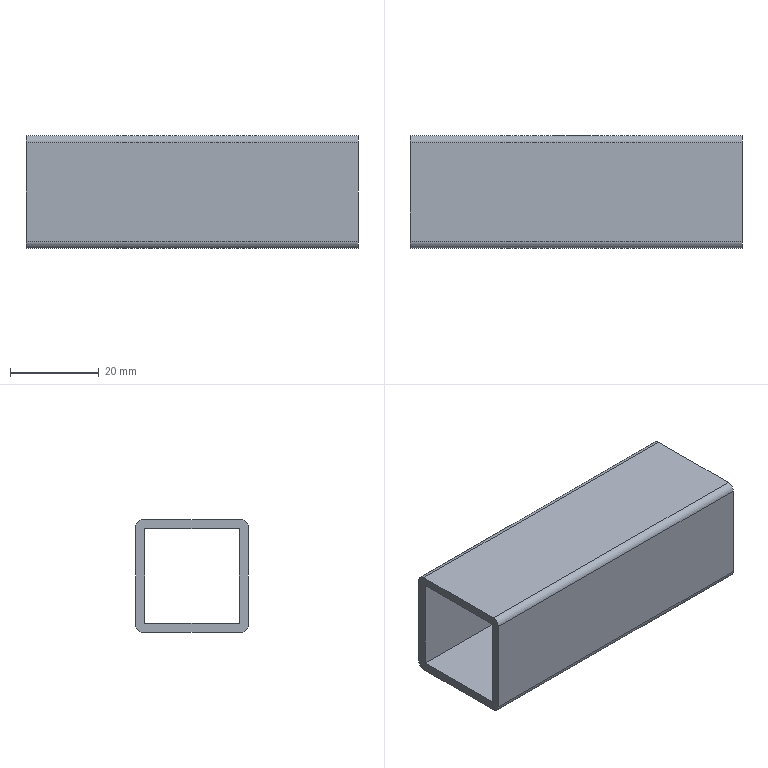Part | NX | features BREP 1 | 1 solid | 16 faces | box 74.93 x 25.4 x 25.4 mm | volume 13599 mm3 | plane 10 | cylinder 6 | commonest cylinder face diameters 3.175 x4 9.652 x2
STEP:
#1=CARTESIAN_POINT('',(-37.465,12.7,-11.113));
#2=VERTEX_POINT('',#1);
#3=CARTESIAN_POINT('',(-37.465,12.7,11.113));
#4=VERTEX_POINT('',#3);
#5=CARTESIAN_POINT('',(-37.465,12.7,-11.113));
#6=DIRECTION('',(0.,0.,1.));
#7=VECTOR('',#6,1000.);
#8=LINE('',#5,#7);
#9=EDGE_CURVE('',#2,#4,#8,.T.);
#10=ORIENTED_EDGE('',*,*,#9,.F.);
#11=CARTESIAN_POINT('',(-37.465,11.113,-12.7));
#12=VERTEX_POINT('',#11);
#13=CARTESIAN_POINT('',(-37.465,11.113,-11.113));
#14=DIRECTION('',(-1.,0.,0.));
#15=DIRECTION('',(0.,1.,0.));
#16=AXIS2_PLACEMENT_3D('',#13,#14,#15);
#17=CIRCLE('',#16,1.587);
#18=EDGE_CURVE('',#2,#12,#17,.T.);
#19=ORIENTED_EDGE('',*,*,#18,.T.);
#20=CARTESIAN_POINT('',(-37.465,-11.113,-12.7));
#21=VERTEX_POINT('',#20);
#22=CARTESIAN_POINT('',(-37.465,-11.113,-12.7));
#23=DIRECTION('',(0.,1.,0.));
#24=VECTOR('',#23,1000.);
#25=LINE('',#22,#24);
#26=EDGE_CURVE('',#21,#12,#25,.T.);
#27=ORIENTED_EDGE('',*,*,#26,.F.);
#28=CARTESIAN_POINT('',(-37.465,-12.7,-11.113));
#29=VERTEX_POINT('',#28);
#30=CARTESIAN_POINT('',(-37.465,-11.113,-11.113));
#31=DIRECTION('',(-1.,0.,0.));
#32=DIRECTION('',(0.,0.,-1.));
#33=AXIS2_PLACEMENT_3D('',#30,#31,#32);
#34=CIRCLE('',#33,1.587);
#35=EDGE_CURVE('',#21,#29,#34,.T.);
#36=ORIENTED_EDGE('',*,*,#35,.T.);
#37=CARTESIAN_POINT('',(-37.465,-12.7,11.113));
#38=VERTEX_POINT('',#37);
#39=CARTESIAN_POINT('',(-37.465,-12.7,11.113));
#40=DIRECTION('',(0.,0.,-1.));
#41=VECTOR('',#40,1000.);
#42=LINE('',#39,#41);
#43=EDGE_CURVE('',#38,#29,#42,.T.);
#44=ORIENTED_EDGE('',*,*,#43,.F.);
#45=CARTESIAN_POINT('',(-37.465,-11.113,12.7));
#46=VERTEX_POINT('',#45);
#47=CARTESIAN_POINT('',(-37.465,-11.113,11.113));
#48=DIRECTION('',(-1.,0.,0.));
#49=DIRECTION('',(0.,-1.,0.));
#50=AXIS2_PLACEMENT_3D('',#47,#48,#49);
#51=CIRCLE('',#50,1.587);
#52=EDGE_CURVE('',#38,#46,#51,.T.);
#53=ORIENTED_EDGE('',*,*,#52,.T.);
#54=CARTESIAN_POINT('',(-37.465,11.113,12.7));
#55=VERTEX_POINT('',#54);
#56=CARTESIAN_POINT('',(-37.465,11.113,12.7));
#57=DIRECTION('',(0.,-1.,0.));
#58=VECTOR('',#57,1000.);
#59=LINE('',#56,#58);
#60=EDGE_CURVE('',#55,#46,#59,.T.);
#61=ORIENTED_EDGE('',*,*,#60,.F.);
#62=CARTESIAN_POINT('',(-37.465,11.113,11.113));
#63=DIRECTION('',(-1.,0.,0.));
#64=DIRECTION('',(0.,0.,1.));
#65=AXIS2_PLACEMENT_3D('',#62,#63,#64);
#66=CIRCLE('',#65,1.587);
#67=EDGE_CURVE('',#55,#4,#66,.T.);
#68=ORIENTED_EDGE('',*,*,#67,.T.);
#69=EDGE_LOOP('',(#10,#19,#27,#36,#44,#53,#61,#68));
#70=FACE_BOUND('',#69,.T.);
#71=CARTESIAN_POINT('',(-37.465,10.719,10.719));
#72=VERTEX_POINT('',#71);
#73=CARTESIAN_POINT('',(-37.465,10.719,-10.719));
#74=VERTEX_POINT('',#73);
#75=CARTESIAN_POINT('',(-37.465,10.719,10.719));
#76=DIRECTION('',(0.,0.,-1.));
#77=VECTOR('',#76,1000.);
#78=LINE('',#75,#77);
#79=EDGE_CURVE('',#72,#74,#78,.T.);
#80=ORIENTED_EDGE('',*,*,#79,.F.);
#81=CARTESIAN_POINT('',(-37.465,-10.719,10.719));
#82=VERTEX_POINT('',#81);
#83=CARTESIAN_POINT('',(-37.465,-10.719,10.719));
#84=DIRECTION('',(0.,1.,0.));
#85=VECTOR('',#84,1000.);
#86=LINE('',#83,#85);
#87=EDGE_CURVE('',#82,#72,#86,.T.);
#88=ORIENTED_EDGE('',*,*,#87,.F.);
#89=CARTESIAN_POINT('',(-37.465,-10.719,-10.719));
#90=VERTEX_POINT('',#89);
#91=CARTESIAN_POINT('',(-37.465,-10.719,-10.719));
#92=DIRECTION('',(0.,0.,1.));
#93=VECTOR('',#92,1000.);
#94=LINE('',#91,#93);
#95=EDGE_CURVE('',#90,#82,#94,.T.);
#96=ORIENTED_EDGE('',*,*,#95,.F.);
#97=CARTESIAN_POINT('',(-37.465,10.719,-10.719));
#98=DIRECTION('',(0.,-1.,0.));
#99=VECTOR('',#98,1000.);
#100=LINE('',#97,#99);
#101=EDGE_CURVE('',#74,#90,#100,.T.);
#102=ORIENTED_EDGE('',*,*,#101,.F.);
#103=EDGE_LOOP('',(#80,#88,#96,#102));
#104=FACE_BOUND('',#103,.T.);
#105=CARTESIAN_POINT('',(-37.465,0.,0.));
#106=DIRECTION('',(1.,0.,0.));
#107=DIRECTION('',(0.,1.,0.));
#108=AXIS2_PLACEMENT_3D('',#105,#106,#107);
#109=PLANE('',#108);
#110=ADVANCED_FACE('',(#70,#104),#109,.F.);
#111=CARTESIAN_POINT('',(37.465,-10.719,-10.719));
#112=VERTEX_POINT('',#111);
#113=CARTESIAN_POINT('',(-37.465,-10.719,-10.719));
#114=DIRECTION('',(1.,0.,0.));
#115=VECTOR('',#114,1000.);
#116=LINE('',#113,#115);
#117=EDGE_CURVE('',#90,#112,#116,.T.);
#118=ORIENTED_EDGE('',*,*,#117,.T.);
#119=CARTESIAN_POINT('',(37.465,10.719,-10.719));
#120=VERTEX_POINT('',#119);
#121=CARTESIAN_POINT('',(37.465,10.719,-10.719));
#122=DIRECTION('',(0.,-1.,0.));
#123=VECTOR('',#122,1000.);
#124=LINE('',#121,#123);
#125=EDGE_CURVE('',#120,#112,#124,.T.);
#126=ORIENTED_EDGE('',*,*,#125,.F.);
#127=CARTESIAN_POINT('',(-37.465,10.719,-10.719));
#128=DIRECTION('',(1.,0.,0.));
#129=VECTOR('',#128,1000.);
#130=LINE('',#127,#129);
#131=EDGE_CURVE('',#74,#120,#130,.T.);
#132=ORIENTED_EDGE('',*,*,#131,.F.);
#133=ORIENTED_EDGE('',*,*,#101,.T.);
#134=EDGE_LOOP('',(#118,#126,#132,#133));
#135=FACE_BOUND('',#134,.T.);
#136=CARTESIAN_POINT('',(-37.465,10.719,-10.719));
#137=DIRECTION('',(0.,0.,1.));
#138=DIRECTION('',(1.,0.,0.));
#139=AXIS2_PLACEMENT_3D('',#136,#137,#138);
#140=PLANE('',#139);
#141=ADVANCED_FACE('',(#135),#140,.T.);
#142=ORIENTED_EDGE('',*,*,#131,.T.);
#143=CARTESIAN_POINT('',(37.465,10.719,10.719));
#144=VERTEX_POINT('',#143);
#145=CARTESIAN_POINT('',(37.465,10.719,10.719));
#146=DIRECTION('',(0.,0.,-1.));
#147=VECTOR('',#146,1000.);
#148=LINE('',#145,#147);
#149=EDGE_CURVE('',#144,#120,#148,.T.);
#150=ORIENTED_EDGE('',*,*,#149,.F.);
#151=CARTESIAN_POINT('',(-37.465,10.719,10.719));
#152=DIRECTION('',(1.,0.,0.));
#153=VECTOR('',#152,1000.);
#154=LINE('',#151,#153);
#155=EDGE_CURVE('',#72,#144,#154,.T.);
#156=ORIENTED_EDGE('',*,*,#155,.F.);
#157=ORIENTED_EDGE('',*,*,#79,.T.);
#158=EDGE_LOOP('',(#142,#150,#156,#157));
#159=FACE_BOUND('',#158,.T.);
#160=CARTESIAN_POINT('',(-4.826,10.719,0.));
#161=VERTEX_POINT('',#160);
#162=CARTESIAN_POINT('',(4.826,10.719,0.));
#163=VERTEX_POINT('',#162);
#164=CARTESIAN_POINT('',(0.,10.719,0.));
#165=DIRECTION('',(0.,-1.,0.));
#166=DIRECTION('',(-1.,0.,0.));
#167=AXIS2_PLACEMENT_3D('',#164,#165,#166);
#168=CIRCLE('',#167,4.826);
#169=EDGE_CURVE('',#161,#163,#168,.T.);
#170=ORIENTED_EDGE('',*,*,#169,.F.);
#171=CARTESIAN_POINT('',(0.,10.719,0.));
#172=DIRECTION('',(0.,-1.,0.));
#173=DIRECTION('',(1.,0.,0.));
#174=AXIS2_PLACEMENT_3D('',#171,#172,#173);
#175=CIRCLE('',#174,4.826);
#176=EDGE_CURVE('',#163,#161,#175,.T.);
#177=ORIENTED_EDGE('',*,*,#176,.F.);
#178=EDGE_LOOP('',(#170,#177));
#179=FACE_BOUND('',#178,.T.);
#180=CARTESIAN_POINT('',(-37.465,10.719,10.719));
#181=DIRECTION('',(0.,-1.,0.));
#182=DIRECTION('',(0.,0.,-1.));
#183=AXIS2_PLACEMENT_3D('',#180,#181,#182);
#184=PLANE('',#183);
#185=ADVANCED_FACE('',(#159,#179),#184,.T.);
#186=ORIENTED_EDGE('',*,*,#155,.T.);
#187=CARTESIAN_POINT('',(37.465,-10.719,10.719));
#188=VERTEX_POINT('',#187);
#189=CARTESIAN_POINT('',(37.465,-10.719,10.719));
#190=DIRECTION('',(0.,1.,0.));
#191=VECTOR('',#190,1000.);
#192=LINE('',#189,#191);
#193=EDGE_CURVE('',#188,#144,#192,.T.);
#194=ORIENTED_EDGE('',*,*,#193,.F.);
#195=CARTESIAN_POINT('',(-37.465,-10.719,10.719));
#196=DIRECTION('',(1.,0.,0.));
#197=VECTOR('',#196,1000.);
#198=LINE('',#195,#197);
#199=EDGE_CURVE('',#82,#188,#198,.T.);
#200=ORIENTED_EDGE('',*,*,#199,.F.);
#201=ORIENTED_EDGE('',*,*,#87,.T.);
#202=EDGE_LOOP('',(#186,#194,#200,#201));
#203=FACE_BOUND('',#202,.T.);
#204=CARTESIAN_POINT('',(-37.465,-10.719,10.719));
#205=DIRECTION('',(0.,0.,-1.));
#206=DIRECTION('',(0.,-1.,0.));
#207=AXIS2_PLACEMENT_3D('',#204,#205,#206);
#208=PLANE('',#207);
#209=ADVANCED_FACE('',(#203),#208,.T.);
#210=ORIENTED_EDGE('',*,*,#199,.T.);
#211=CARTESIAN_POINT('',(37.465,-10.719,-10.719));
#212=DIRECTION('',(0.,0.,1.));
#213=VECTOR('',#212,1000.);
#214=LINE('',#211,#213);
#215=EDGE_CURVE('',#112,#188,#214,.T.);
#216=ORIENTED_EDGE('',*,*,#215,.F.);
#217=ORIENTED_EDGE('',*,*,#117,.F.);
#218=ORIENTED_EDGE('',*,*,#95,.T.);
#219=EDGE_LOOP('',(#210,#216,#217,#218));
#220=FACE_BOUND('',#219,.T.);
#221=CARTESIAN_POINT('',(-37.465,-10.719,-10.719));
#222=DIRECTION('',(0.,1.,0.));
#223=DIRECTION('',(1.,0.,0.));
#224=AXIS2_PLACEMENT_3D('',#221,#222,#223);
#225=PLANE('',#224);
#226=ADVANCED_FACE('',(#220),#225,.T.);
#227=CARTESIAN_POINT('',(37.465,11.113,12.7));
#228=VERTEX_POINT('',#227);
#229=CARTESIAN_POINT('',(37.465,-11.113,12.7));
#230=VERTEX_POINT('',#229);
#231=CARTESIAN_POINT('',(37.465,11.113,12.7));
#232=DIRECTION('',(0.,-1.,0.));
#233=VECTOR('',#232,1000.);
#234=LINE('',#231,#233);
#235=EDGE_CURVE('',#228,#230,#234,.T.);
#236=ORIENTED_EDGE('',*,*,#235,.T.);
#237=CARTESIAN_POINT('',(37.465,-12.7,11.113));
#238=VERTEX_POINT('',#237);
#239=CARTESIAN_POINT('',(37.465,-11.113,11.113));
#240=DIRECTION('',(1.,0.,0.));
#241=DIRECTION('',(0.,0.,1.));
#242=AXIS2_PLACEMENT_3D('',#239,#240,#241);
#243=CIRCLE('',#242,1.587);
#244=EDGE_CURVE('',#230,#238,#243,.T.);
#245=ORIENTED_EDGE('',*,*,#244,.T.);
#246=CARTESIAN_POINT('',(37.465,-12.7,-11.113));
#247=VERTEX_POINT('',#246);
#248=CARTESIAN_POINT('',(37.465,-12.7,11.113));
#249=DIRECTION('',(0.,0.,-1.));
#250=VECTOR('',#249,1000.);
#251=LINE('',#248,#250);
#252=EDGE_CURVE('',#238,#247,#251,.T.);
#253=ORIENTED_EDGE('',*,*,#252,.T.);
#254=CARTESIAN_POINT('',(37.465,-11.113,-12.7));
#255=VERTEX_POINT('',#254);
#256=CARTESIAN_POINT('',(37.465,-11.113,-11.113));
#257=DIRECTION('',(1.,0.,0.));
#258=DIRECTION('',(0.,-1.,0.));
#259=AXIS2_PLACEMENT_3D('',#256,#257,#258);
#260=CIRCLE('',#259,1.587);
#261=EDGE_CURVE('',#247,#255,#260,.T.);
#262=ORIENTED_EDGE('',*,*,#261,.T.);
#263=CARTESIAN_POINT('',(37.465,11.113,-12.7));
#264=VERTEX_POINT('',#263);
#265=CARTESIAN_POINT('',(37.465,-11.113,-12.7));
#266=DIRECTION('',(0.,1.,0.));
#267=VECTOR('',#266,1000.);
#268=LINE('',#265,#267);
#269=EDGE_CURVE('',#255,#264,#268,.T.);
#270=ORIENTED_EDGE('',*,*,#269,.T.);
#271=CARTESIAN_POINT('',(37.465,12.7,-11.113));
#272=VERTEX_POINT('',#271);
#273=CARTESIAN_POINT('',(37.465,11.113,-11.113));
#274=DIRECTION('',(1.,0.,0.));
#275=DIRECTION('',(0.,0.,-1.));
#276=AXIS2_PLACEMENT_3D('',#273,#274,#275);
#277=CIRCLE('',#276,1.587);
#278=EDGE_CURVE('',#264,#272,#277,.T.);
#279=ORIENTED_EDGE('',*,*,#278,.T.);
#280=CARTESIAN_POINT('',(37.465,12.7,11.113));
#281=VERTEX_POINT('',#280);
#282=CARTESIAN_POINT('',(37.465,12.7,-11.113));
#283=DIRECTION('',(0.,0.,1.));
#284=VECTOR('',#283,1000.);
#285=LINE('',#282,#284);
#286=EDGE_CURVE('',#272,#281,#285,.T.);
#287=ORIENTED_EDGE('',*,*,#286,.T.);
#288=CARTESIAN_POINT('',(37.465,11.113,11.113));
#289=DIRECTION('',(1.,0.,0.));
#290=DIRECTION('',(0.,1.,0.));
#291=AXIS2_PLACEMENT_3D('',#288,#289,#290);
#292=CIRCLE('',#291,1.587);
#293=EDGE_CURVE('',#281,#228,#292,.T.);
#294=ORIENTED_EDGE('',*,*,#293,.T.);
#295=EDGE_LOOP('',(#236,#245,#253,#262,#270,#279,#287,#294));
#296=FACE_BOUND('',#295,.T.);
#297=ORIENTED_EDGE('',*,*,#215,.T.);
#298=ORIENTED_EDGE('',*,*,#193,.T.);
#299=ORIENTED_EDGE('',*,*,#149,.T.);
#300=ORIENTED_EDGE('',*,*,#125,.T.);
#301=EDGE_LOOP('',(#297,#298,#299,#300));
#302=FACE_BOUND('',#301,.T.);
#303=CARTESIAN_POINT('',(37.465,0.,0.));
#304=DIRECTION('',(1.,0.,0.));
#305=DIRECTION('',(0.,1.,0.));
#306=AXIS2_PLACEMENT_3D('',#303,#304,#305);
#307=PLANE('',#306);
#308=ADVANCED_FACE('',(#296,#302),#307,.T.);
#309=ORIENTED_EDGE('',*,*,#293,.F.);
#310=CARTESIAN_POINT('',(37.465,12.7,11.113));
#311=DIRECTION('',(-1.,0.,0.));
#312=VECTOR('',#311,1000.);
#313=LINE('',#310,#312);
#314=EDGE_CURVE('',#281,#4,#313,.T.);
#315=ORIENTED_EDGE('',*,*,#314,.T.);
#316=ORIENTED_EDGE('',*,*,#67,.F.);
#317=CARTESIAN_POINT('',(37.465,11.113,12.7));
#318=DIRECTION('',(-1.,0.,0.));
#319=VECTOR('',#318,1000.);
#320=LINE('',#317,#319);
#321=EDGE_CURVE('',#228,#55,#320,.T.);
#322=ORIENTED_EDGE('',*,*,#321,.F.);
#323=EDGE_LOOP('',(#309,#315,#316,#322));
#324=FACE_BOUND('',#323,.T.);
#325=CARTESIAN_POINT('',(37.595,11.113,11.113));
#326=DIRECTION('',(-1.,0.,0.));
#327=DIRECTION('',(0.,0.,1.));
#328=AXIS2_PLACEMENT_3D('',#325,#326,#327);
#329=CYLINDRICAL_SURFACE('',#328,1.587);
#330=ADVANCED_FACE('',(#324),#329,.T.);
#331=ORIENTED_EDGE('',*,*,#60,.T.);
#332=CARTESIAN_POINT('',(37.465,-11.113,12.7));
#333=DIRECTION('',(-1.,0.,0.));
#334=VECTOR('',#333,1000.);
#335=LINE('',#332,#334);
#336=EDGE_CURVE('',#230,#46,#335,.T.);
#337=ORIENTED_EDGE('',*,*,#336,.F.);
#338=ORIENTED_EDGE('',*,*,#235,.F.);
#339=ORIENTED_EDGE('',*,*,#321,.T.);
#340=EDGE_LOOP('',(#331,#337,#338,#339));
#341=FACE_BOUND('',#340,.T.);
#342=CARTESIAN_POINT('',(-37.465,12.7,12.7));
#343=DIRECTION('',(0.,0.,1.));
#344=DIRECTION('',(1.,0.,0.));
#345=AXIS2_PLACEMENT_3D('',#342,#343,#344);
#346=PLANE('',#345);
#347=ADVANCED_FACE('',(#341),#346,.T.);
#348=ORIENTED_EDGE('',*,*,#244,.F.);
#349=ORIENTED_EDGE('',*,*,#336,.T.);
#350=ORIENTED_EDGE('',*,*,#52,.F.);
#351=CARTESIAN_POINT('',(37.465,-12.7,11.113));
#352=DIRECTION('',(-1.,0.,0.));
#353=VECTOR('',#352,1000.);
#354=LINE('',#351,#353);
#355=EDGE_CURVE('',#238,#38,#354,.T.);
#356=ORIENTED_EDGE('',*,*,#355,.F.);
#357=EDGE_LOOP('',(#348,#349,#350,#356));
#358=FACE_BOUND('',#357,.T.);
#359=CARTESIAN_POINT('',(37.595,-11.113,11.113));
#360=DIRECTION('',(-1.,0.,0.));
#361=DIRECTION('',(0.,-1.,0.));
#362=AXIS2_PLACEMENT_3D('',#359,#360,#361);
#363=CYLINDRICAL_SURFACE('',#362,1.587);
#364=ADVANCED_FACE('',(#358),#363,.T.);
#365=ORIENTED_EDGE('',*,*,#43,.T.);
#366=CARTESIAN_POINT('',(37.465,-12.7,-11.113));
#367=DIRECTION('',(-1.,0.,0.));
#368=VECTOR('',#367,1000.);
#369=LINE('',#366,#368);
#370=EDGE_CURVE('',#247,#29,#369,.T.);
#371=ORIENTED_EDGE('',*,*,#370,.F.);
#372=ORIENTED_EDGE('',*,*,#252,.F.);
#373=ORIENTED_EDGE('',*,*,#355,.T.);
#374=EDGE_LOOP('',(#365,#371,#372,#373));
#375=FACE_BOUND('',#374,.T.);
#376=CARTESIAN_POINT('',(-37.465,-12.7,12.7));
#377=DIRECTION('',(0.,-1.,0.));
#378=DIRECTION('',(0.,0.,-1.));
#379=AXIS2_PLACEMENT_3D('',#376,#377,#378);
#380=PLANE('',#379);
#381=ADVANCED_FACE('',(#375),#380,.T.);
#382=ORIENTED_EDGE('',*,*,#261,.F.);
#383=ORIENTED_EDGE('',*,*,#370,.T.);
#384=ORIENTED_EDGE('',*,*,#35,.F.);
#385=CARTESIAN_POINT('',(37.465,-11.113,-12.7));
#386=DIRECTION('',(-1.,0.,0.));
#387=VECTOR('',#386,1000.);
#388=LINE('',#385,#387);
#389=EDGE_CURVE('',#255,#21,#388,.T.);
#390=ORIENTED_EDGE('',*,*,#389,.F.);
#391=EDGE_LOOP('',(#382,#383,#384,#390));
#392=FACE_BOUND('',#391,.T.);
#393=CARTESIAN_POINT('',(37.595,-11.113,-11.113));
#394=DIRECTION('',(-1.,0.,0.));
#395=DIRECTION('',(0.,0.,-1.));
#396=AXIS2_PLACEMENT_3D('',#393,#394,#395);
#397=CYLINDRICAL_SURFACE('',#396,1.587);
#398=ADVANCED_FACE('',(#392),#397,.T.);
#399=ORIENTED_EDGE('',*,*,#269,.F.);
#400=ORIENTED_EDGE('',*,*,#389,.T.);
#401=ORIENTED_EDGE('',*,*,#26,.T.);
#402=CARTESIAN_POINT('',(37.465,11.113,-12.7));
#403=DIRECTION('',(-1.,0.,0.));
#404=VECTOR('',#403,1000.);
#405=LINE('',#402,#404);
#406=EDGE_CURVE('',#264,#12,#405,.T.);
#407=ORIENTED_EDGE('',*,*,#406,.F.);
#408=EDGE_LOOP('',(#399,#400,#401,#407));
#409=FACE_BOUND('',#408,.T.);
#410=CARTESIAN_POINT('',(-37.465,-12.7,-12.7));
#411=DIRECTION('',(0.,0.,-1.));
#412=DIRECTION('',(0.,-1.,0.));
#413=AXIS2_PLACEMENT_3D('',#410,#411,#412);
#414=PLANE('',#413);
#415=ADVANCED_FACE('',(#409),#414,.T.);
#416=ORIENTED_EDGE('',*,*,#278,.F.);
#417=ORIENTED_EDGE('',*,*,#406,.T.);
#418=ORIENTED_EDGE('',*,*,#18,.F.);
#419=CARTESIAN_POINT('',(37.465,12.7,-11.113));
#420=DIRECTION('',(-1.,0.,0.));
#421=VECTOR('',#420,1000.);
#422=LINE('',#419,#421);
#423=EDGE_CURVE('',#272,#2,#422,.T.);
#424=ORIENTED_EDGE('',*,*,#423,.F.);
#425=EDGE_LOOP('',(#416,#417,#418,#424));
#426=FACE_BOUND('',#425,.T.);
#427=CARTESIAN_POINT('',(37.595,11.113,-11.113));
#428=DIRECTION('',(-1.,0.,0.));
#429=DIRECTION('',(0.,1.,0.));
#430=AXIS2_PLACEMENT_3D('',#427,#428,#429);
#431=CYLINDRICAL_SURFACE('',#430,1.587);
#432=ADVANCED_FACE('',(#426),#431,.T.);
#433=ORIENTED_EDGE('',*,*,#286,.F.);
#434=ORIENTED_EDGE('',*,*,#423,.T.);
#435=ORIENTED_EDGE('',*,*,#9,.T.);
#436=ORIENTED_EDGE('',*,*,#314,.F.);
#437=EDGE_LOOP('',(#433,#434,#435,#436));
#438=FACE_BOUND('',#437,.T.);
#439=CARTESIAN_POINT('',(-4.826,12.7,0.));
#440=VERTEX_POINT('',#439);
#441=CARTESIAN_POINT('',(4.826,12.7,0.));
#442=VERTEX_POINT('',#441);
#443=CARTESIAN_POINT('',(0.,12.7,0.));
#444=DIRECTION('',(0.,-1.,0.));
#445=DIRECTION('',(-1.,0.,0.));
#446=AXIS2_PLACEMENT_3D('',#443,#444,#445);
#447=CIRCLE('',#446,4.826);
#448=EDGE_CURVE('',#440,#442,#447,.T.);
#449=ORIENTED_EDGE('',*,*,#448,.T.);
#450=CARTESIAN_POINT('',(0.,12.7,0.));
#451=DIRECTION('',(0.,-1.,0.));
#452=DIRECTION('',(1.,0.,0.));
#453=AXIS2_PLACEMENT_3D('',#450,#451,#452);
#454=CIRCLE('',#453,4.826);
#455=EDGE_CURVE('',#442,#440,#454,.T.);
#456=ORIENTED_EDGE('',*,*,#455,.T.);
#457=EDGE_LOOP('',(#449,#456));
#458=FACE_BOUND('',#457,.T.);
#459=CARTESIAN_POINT('',(-37.465,12.7,-12.7));
#460=DIRECTION('',(0.,1.,0.));
#461=DIRECTION('',(1.,0.,0.));
#462=AXIS2_PLACEMENT_3D('',#459,#460,#461);
#463=PLANE('',#462);
#464=ADVANCED_FACE('',(#438,#458),#463,.T.);
#465=CARTESIAN_POINT('',(4.826,12.7,0.));
#466=DIRECTION('',(0.,-1.,0.));
#467=VECTOR('',#466,1000.);
#468=LINE('',#465,#467);
#469=EDGE_CURVE('',#163,#442,#468,.F.);
#470=ORIENTED_EDGE('',*,*,#469,.F.);
#471=ORIENTED_EDGE('',*,*,#176,.T.);
#472=CARTESIAN_POINT('',(-4.826,12.7,0.));
#473=DIRECTION('',(0.,-1.,0.));
#474=VECTOR('',#473,1000.);
#475=LINE('',#472,#474);
#476=EDGE_CURVE('',#161,#440,#475,.F.);
#477=ORIENTED_EDGE('',*,*,#476,.T.);
#478=ORIENTED_EDGE('',*,*,#455,.F.);
#479=EDGE_LOOP('',(#470,#471,#477,#478));
#480=FACE_BOUND('',#479,.T.);
#481=CARTESIAN_POINT('',(0.,12.7,0.));
#482=DIRECTION('',(0.,-1.,0.));
#483=DIRECTION('',(1.,0.,0.));
#484=AXIS2_PLACEMENT_3D('',#481,#482,#483);
#485=CYLINDRICAL_SURFACE('',#484,4.826);
#486=ADVANCED_FACE('',(#480),#485,.F.);
#487=ORIENTED_EDGE('',*,*,#476,.F.);
#488=ORIENTED_EDGE('',*,*,#169,.T.);
#489=ORIENTED_EDGE('',*,*,#469,.T.);
#490=ORIENTED_EDGE('',*,*,#448,.F.);
#491=EDGE_LOOP('',(#487,#488,#489,#490));
#492=FACE_BOUND('',#491,.T.);
#493=CARTESIAN_POINT('',(0.,12.7,0.));
#494=DIRECTION('',(0.,-1.,0.));
#495=DIRECTION('',(1.,0.,0.));
#496=AXIS2_PLACEMENT_3D('',#493,#494,#495);
#497=CYLINDRICAL_SURFACE('',#496,4.826);
#498=ADVANCED_FACE('',(#492),#497,.F.);
#499=CLOSED_SHELL('',(#110,#141,#185,#209,#226,#308,#330,#347,#364,#381,#398,#415,#432,#464,#486,#498));
#500=MANIFOLD_SOLID_BREP('',#499);
#501=(LENGTH_UNIT()NAMED_UNIT(*)SI_UNIT(.MILLI.,.METRE.));
#502=UNCERTAINTY_MEASURE_WITH_UNIT(LENGTH_MEASURE(0.00001),#501,'','');
#503=(NAMED_UNIT(*)PLANE_ANGLE_UNIT()SI_UNIT($,.RADIAN.));
#504=(NAMED_UNIT(*)SI_UNIT($,.STERADIAN.)SOLID_ANGLE_UNIT());
#505=(GEOMETRIC_REPRESENTATION_CONTEXT(3)GLOBAL_UNCERTAINTY_ASSIGNED_CONTEXT((#502))GLOBAL_UNIT_ASSIGNED_CONTEXT((#501,#503,#504))REPRESENTATION_CONTEXT('',''));
#506=ADVANCED_BREP_SHAPE_REPRESENTATION('',(#500),#505);